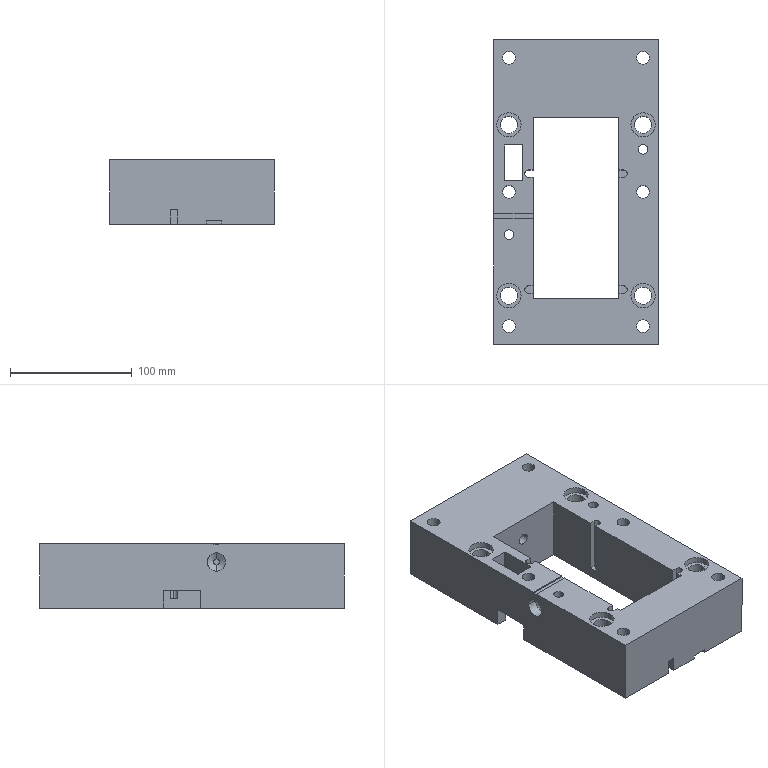Part | STEP file | KHUON BAO TREN_2 | 1 solid | 117 faces | box 135 x 250 x 53 mm | volume 1110961 mm3 | cylinder 63 | plane 52 | cone 2 | commonest cylinder face diameters 16 x13 10.5 x12 6 x8 14 x8 20 x8 1 x4